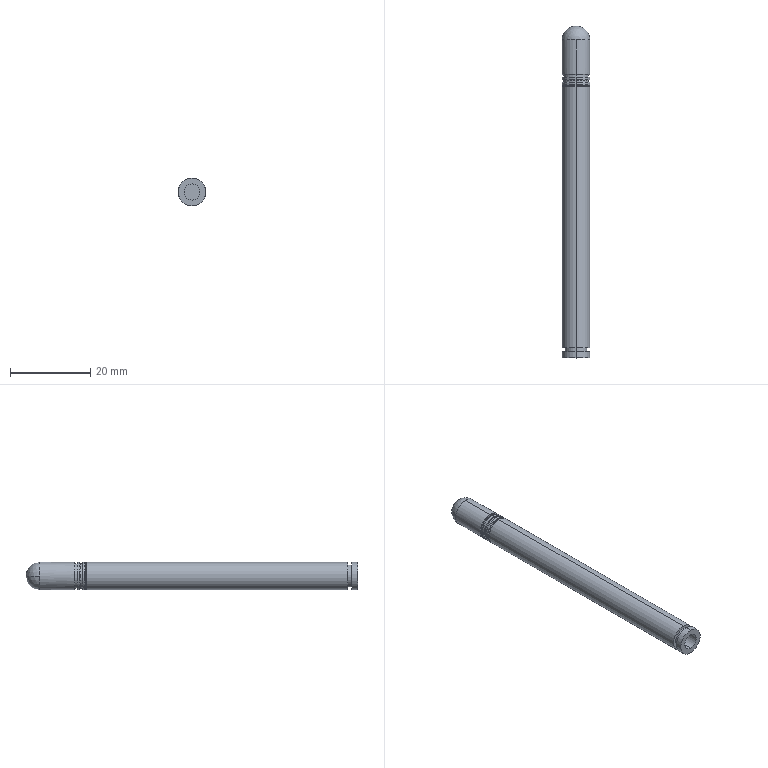Part | SolidWorks | features Revolution 1 | 1 solid | 56 faces | box 6.9 x 82.6 x 6.9 mm | volume 2024 mm3 | torus 24 | cylinder 20 | plane 10 | sphere 2 | commonest cylinder face diameters 6.9 x10 6.2 x6 4 x2 5.4 x2
STEP:
#1=CARTESIAN_POINT('',(0.,2.7,-2.7));
#2=VERTEX_POINT('',#1);
#3=CARTESIAN_POINT('',(0.,2.7,2.7));
#4=VERTEX_POINT('',#3);
#5=CARTESIAN_POINT('',(0.,2.7,0.));
#6=DIRECTION('',(0.,-1.,0.));
#7=DIRECTION('',(0.,0.,-1.));
#8=AXIS2_PLACEMENT_3D('',#5,#6,#7);
#9=CIRCLE('',#8,2.7);
#10=EDGE_CURVE('',#2,#4,#9,.T.);
#11=ORIENTED_EDGE('',*,*,#10,.T.);
#12=CARTESIAN_POINT('',(0.,1.7,2.7));
#13=VERTEX_POINT('',#12);
#14=CARTESIAN_POINT('',(0.,-7.874,2.7));
#15=DIRECTION('',(0.,-1.,0.));
#16=VECTOR('',#15,1000.);
#17=LINE('',#14,#16);
#18=EDGE_CURVE('',#4,#13,#17,.T.);
#19=ORIENTED_EDGE('',*,*,#18,.T.);
#20=CARTESIAN_POINT('',(0.,1.7,-2.7));
#21=VERTEX_POINT('',#20);
#22=CARTESIAN_POINT('',(0.,1.7,0.));
#23=DIRECTION('',(0.,-1.,0.));
#24=DIRECTION('',(0.,0.,-1.));
#25=AXIS2_PLACEMENT_3D('',#22,#23,#24);
#26=CIRCLE('',#25,2.7);
#27=EDGE_CURVE('',#21,#13,#26,.T.);
#28=ORIENTED_EDGE('',*,*,#27,.F.);
#29=CARTESIAN_POINT('',(0.,-7.874,-2.7));
#30=DIRECTION('',(0.,-1.,0.));
#31=VECTOR('',#30,1000.);
#32=LINE('',#29,#31);
#33=EDGE_CURVE('',#2,#21,#32,.T.);
#34=ORIENTED_EDGE('',*,*,#33,.F.);
#35=EDGE_LOOP('',(#11,#19,#28,#34));
#36=FACE_OUTER_BOUND('',#35,.T.);
#37=CARTESIAN_POINT('',(0.,-7.874,0.));
#38=DIRECTION('',(0.,-1.,0.));
#39=DIRECTION('',(0.,0.,-1.));
#40=AXIS2_PLACEMENT_3D('',#37,#38,#39);
#41=CYLINDRICAL_SURFACE('',#40,2.7);
#42=ADVANCED_FACE('',(#36),#41,.T.);
#43=CARTESIAN_POINT('',(0.,67.65,-3.45));
#44=VERTEX_POINT('',#43);
#45=CARTESIAN_POINT('',(0.,67.65,3.45));
#46=VERTEX_POINT('',#45);
#47=CARTESIAN_POINT('',(0.,67.65,0.));
#48=DIRECTION('',(0.,-1.,0.));
#49=DIRECTION('',(0.,0.,-1.));
#50=AXIS2_PLACEMENT_3D('',#47,#48,#49);
#51=CIRCLE('',#50,3.45);
#52=EDGE_CURVE('',#44,#46,#51,.T.);
#53=ORIENTED_EDGE('',*,*,#52,.T.);
#54=CARTESIAN_POINT('',(0.,2.7,3.45));
#55=VERTEX_POINT('',#54);
#56=CARTESIAN_POINT('',(0.,-7.874,3.45));
#57=DIRECTION('',(0.,-1.,0.));
#58=VECTOR('',#57,1000.);
#59=LINE('',#56,#58);
#60=EDGE_CURVE('',#46,#55,#59,.T.);
#61=ORIENTED_EDGE('',*,*,#60,.T.);
#62=CARTESIAN_POINT('',(0.,2.7,-3.45));
#63=VERTEX_POINT('',#62);
#64=CARTESIAN_POINT('',(0.,2.7,0.));
#65=DIRECTION('',(0.,-1.,0.));
#66=DIRECTION('',(0.,0.,-1.));
#67=AXIS2_PLACEMENT_3D('',#64,#65,#66);
#68=CIRCLE('',#67,3.45);
#69=EDGE_CURVE('',#63,#55,#68,.T.);
#70=ORIENTED_EDGE('',*,*,#69,.F.);
#71=CARTESIAN_POINT('',(0.,-7.874,-3.45));
#72=DIRECTION('',(0.,-1.,0.));
#73=VECTOR('',#72,1000.);
#74=LINE('',#71,#73);
#75=EDGE_CURVE('',#44,#63,#74,.T.);
#76=ORIENTED_EDGE('',*,*,#75,.F.);
#77=EDGE_LOOP('',(#53,#61,#70,#76));
#78=FACE_OUTER_BOUND('',#77,.T.);
#79=CARTESIAN_POINT('',(0.,-7.874,0.));
#80=DIRECTION('',(0.,-1.,0.));
#81=DIRECTION('',(0.,0.,-1.));
#82=AXIS2_PLACEMENT_3D('',#79,#80,#81);
#83=CYLINDRICAL_SURFACE('',#82,3.45);
#84=ADVANCED_FACE('',(#78),#83,.T.);
#85=CARTESIAN_POINT('',(0.,67.7,-3.4));
#86=VERTEX_POINT('',#85);
#87=CARTESIAN_POINT('',(0.,67.7,3.4));
#88=VERTEX_POINT('',#87);
#89=CARTESIAN_POINT('',(0.,67.7,0.));
#90=DIRECTION('',(0.,-1.,0.));
#91=DIRECTION('',(0.,0.,-1.));
#92=AXIS2_PLACEMENT_3D('',#89,#90,#91);
#93=CIRCLE('',#92,3.4);
#94=EDGE_CURVE('',#86,#88,#93,.T.);
#95=ORIENTED_EDGE('',*,*,#94,.T.);
#96=CARTESIAN_POINT('',(0.,67.65,3.4));
#97=DIRECTION('',(1.,0.,0.));
#98=DIRECTION('',(0.,0.,-1.));
#99=AXIS2_PLACEMENT_3D('',#96,#97,#98);
#100=CIRCLE('',#99,0.05);
#101=EDGE_CURVE('',#88,#46,#100,.T.);
#102=ORIENTED_EDGE('',*,*,#101,.T.);
#103=ORIENTED_EDGE('',*,*,#52,.F.);
#104=CARTESIAN_POINT('',(0.,67.65,-3.4));
#105=DIRECTION('',(-1.,0.,0.));
#106=DIRECTION('',(0.,0.,1.));
#107=AXIS2_PLACEMENT_3D('',#104,#105,#106);
#108=CIRCLE('',#107,0.05);
#109=EDGE_CURVE('',#86,#44,#108,.T.);
#110=ORIENTED_EDGE('',*,*,#109,.F.);
#111=EDGE_LOOP('',(#95,#102,#103,#110));
#112=FACE_OUTER_BOUND('',#111,.T.);
#113=CARTESIAN_POINT('',(0.,67.65,0.));
#114=DIRECTION('',(0.,-1.,0.));
#115=DIRECTION('',(0.,0.,-1.));
#116=AXIS2_PLACEMENT_3D('',#113,#114,#115);
#117=TOROIDAL_SURFACE('',#116,3.4,0.05);
#118=ADVANCED_FACE('',(#112),#117,.T.);
#119=CARTESIAN_POINT('',(0.,67.7,3.15));
#120=VERTEX_POINT('',#119);
#121=CARTESIAN_POINT('',(0.,67.7,-3.15));
#122=VERTEX_POINT('',#121);
#123=CARTESIAN_POINT('',(0.,67.7,0.));
#124=DIRECTION('',(0.,-1.,0.));
#125=DIRECTION('',(0.,0.,-1.));
#126=AXIS2_PLACEMENT_3D('',#123,#124,#125);
#127=CIRCLE('',#126,3.15);
#128=EDGE_CURVE('',#120,#122,#127,.T.);
#129=ORIENTED_EDGE('',*,*,#128,.F.);
#130=CARTESIAN_POINT('',(0.,67.75,3.1));
#131=VERTEX_POINT('',#130);
#132=CARTESIAN_POINT('',(0.,67.75,3.15));
#133=DIRECTION('',(1.,0.,0.));
#134=DIRECTION('',(0.,0.,-1.));
#135=AXIS2_PLACEMENT_3D('',#132,#133,#134);
#136=CIRCLE('',#135,0.05);
#137=EDGE_CURVE('',#120,#131,#136,.T.);
#138=ORIENTED_EDGE('',*,*,#137,.T.);
#139=CARTESIAN_POINT('',(0.,67.75,-3.1));
#140=VERTEX_POINT('',#139);
#141=CARTESIAN_POINT('',(0.,67.75,0.));
#142=DIRECTION('',(0.,-1.,0.));
#143=DIRECTION('',(0.,0.,-1.));
#144=AXIS2_PLACEMENT_3D('',#141,#142,#143);
#145=CIRCLE('',#144,3.1);
#146=EDGE_CURVE('',#131,#140,#145,.T.);
#147=ORIENTED_EDGE('',*,*,#146,.T.);
#148=CARTESIAN_POINT('',(0.,67.75,-3.15));
#149=DIRECTION('',(-1.,0.,0.));
#150=DIRECTION('',(0.,0.,1.));
#151=AXIS2_PLACEMENT_3D('',#148,#149,#150);
#152=CIRCLE('',#151,0.05);
#153=EDGE_CURVE('',#122,#140,#152,.T.);
#154=ORIENTED_EDGE('',*,*,#153,.F.);
#155=EDGE_LOOP('',(#129,#138,#147,#154));
#156=FACE_OUTER_BOUND('',#155,.T.);
#157=CARTESIAN_POINT('',(0.,67.75,0.));
#158=DIRECTION('',(0.,-1.,0.));
#159=DIRECTION('',(0.,0.,-1.));
#160=AXIS2_PLACEMENT_3D('',#157,#158,#159);
#161=TOROIDAL_SURFACE('',#160,3.15,0.05);
#162=ADVANCED_FACE('',(#156),#161,.F.);
#163=CARTESIAN_POINT('',(0.,68.05,-3.1));
#164=VERTEX_POINT('',#163);
#165=CARTESIAN_POINT('',(0.,68.05,3.1));
#166=VERTEX_POINT('',#165);
#167=CARTESIAN_POINT('',(0.,68.05,0.));
#168=DIRECTION('',(0.,-1.,0.));
#169=DIRECTION('',(0.,0.,-1.));
#170=AXIS2_PLACEMENT_3D('',#167,#168,#169);
#171=CIRCLE('',#170,3.1);
#172=EDGE_CURVE('',#164,#166,#171,.T.);
#173=ORIENTED_EDGE('',*,*,#172,.T.);
#174=CARTESIAN_POINT('',(0.,-7.874,3.1));
#175=DIRECTION('',(0.,-1.,0.));
#176=VECTOR('',#175,1000.);
#177=LINE('',#174,#176);
#178=EDGE_CURVE('',#166,#131,#177,.T.);
#179=ORIENTED_EDGE('',*,*,#178,.T.);
#180=CARTESIAN_POINT('',(0.,67.75,0.));
#181=DIRECTION('',(0.,-1.,0.));
#182=DIRECTION('',(0.,0.,-1.));
#183=AXIS2_PLACEMENT_3D('',#180,#181,#182);
#184=CIRCLE('',#183,3.1);
#185=EDGE_CURVE('',#140,#131,#184,.T.);
#186=ORIENTED_EDGE('',*,*,#185,.F.);
#187=CARTESIAN_POINT('',(0.,-7.874,-3.1));
#188=DIRECTION('',(0.,-1.,0.));
#189=VECTOR('',#188,1000.);
#190=LINE('',#187,#189);
#191=EDGE_CURVE('',#164,#140,#190,.T.);
#192=ORIENTED_EDGE('',*,*,#191,.F.);
#193=EDGE_LOOP('',(#173,#179,#186,#192));
#194=FACE_OUTER_BOUND('',#193,.T.);
#195=CARTESIAN_POINT('',(0.,-7.874,0.));
#196=DIRECTION('',(0.,-1.,0.));
#197=DIRECTION('',(0.,0.,-1.));
#198=AXIS2_PLACEMENT_3D('',#195,#196,#197);
#199=CYLINDRICAL_SURFACE('',#198,3.1);
#200=ADVANCED_FACE('',(#194),#199,.T.);
#201=CARTESIAN_POINT('',(0.,68.05,0.));
#202=DIRECTION('',(0.,-1.,0.));
#203=DIRECTION('',(0.,0.,-1.));
#204=AXIS2_PLACEMENT_3D('',#201,#202,#203);
#205=CIRCLE('',#204,3.1);
#206=EDGE_CURVE('',#166,#164,#205,.T.);
#207=ORIENTED_EDGE('',*,*,#206,.F.);
#208=CARTESIAN_POINT('',(0.,68.1,3.15));
#209=VERTEX_POINT('',#208);
#210=CARTESIAN_POINT('',(0.,68.05,3.15));
#211=DIRECTION('',(1.,0.,0.));
#212=DIRECTION('',(0.,0.,-1.));
#213=AXIS2_PLACEMENT_3D('',#210,#211,#212);
#214=CIRCLE('',#213,0.05);
#215=EDGE_CURVE('',#166,#209,#214,.T.);
#216=ORIENTED_EDGE('',*,*,#215,.T.);
#217=CARTESIAN_POINT('',(0.,68.1,-3.15));
#218=VERTEX_POINT('',#217);
#219=CARTESIAN_POINT('',(0.,68.1,0.));
#220=DIRECTION('',(0.,-1.,0.));
#221=DIRECTION('',(0.,0.,-1.));
#222=AXIS2_PLACEMENT_3D('',#219,#220,#221);
#223=CIRCLE('',#222,3.15);
#224=EDGE_CURVE('',#209,#218,#223,.T.);
#225=ORIENTED_EDGE('',*,*,#224,.T.);
#226=CARTESIAN_POINT('',(0.,68.05,-3.15));
#227=DIRECTION('',(-1.,0.,0.));
#228=DIRECTION('',(0.,0.,1.));
#229=AXIS2_PLACEMENT_3D('',#226,#227,#228);
#230=CIRCLE('',#229,0.05);
#231=EDGE_CURVE('',#164,#218,#230,.T.);
#232=ORIENTED_EDGE('',*,*,#231,.F.);
#233=EDGE_LOOP('',(#207,#216,#225,#232));
#234=FACE_OUTER_BOUND('',#233,.T.);
#235=CARTESIAN_POINT('',(0.,68.05,0.));
#236=DIRECTION('',(0.,-1.,0.));
#237=DIRECTION('',(0.,0.,-1.));
#238=AXIS2_PLACEMENT_3D('',#235,#236,#237);
#239=TOROIDAL_SURFACE('',#238,3.15,0.05);
#240=ADVANCED_FACE('',(#234),#239,.F.);
#241=CARTESIAN_POINT('',(0.,68.15,-3.45));
#242=VERTEX_POINT('',#241);
#243=CARTESIAN_POINT('',(0.,68.15,3.45));
#244=VERTEX_POINT('',#243);
#245=CARTESIAN_POINT('',(0.,68.15,0.));
#246=DIRECTION('',(0.,-1.,0.));
#247=DIRECTION('',(0.,0.,-1.));
#248=AXIS2_PLACEMENT_3D('',#245,#246,#247);
#249=CIRCLE('',#248,3.45);
#250=EDGE_CURVE('',#242,#244,#249,.T.);
#251=ORIENTED_EDGE('',*,*,#250,.T.);
#252=CARTESIAN_POINT('',(0.,68.1,3.4));
#253=VERTEX_POINT('',#252);
#254=CARTESIAN_POINT('',(0.,68.15,3.4));
#255=DIRECTION('',(1.,0.,0.));
#256=DIRECTION('',(0.,0.,-1.));
#257=AXIS2_PLACEMENT_3D('',#254,#255,#256);
#258=CIRCLE('',#257,0.05);
#259=EDGE_CURVE('',#244,#253,#258,.T.);
#260=ORIENTED_EDGE('',*,*,#259,.T.);
#261=CARTESIAN_POINT('',(0.,68.1,-3.4));
#262=VERTEX_POINT('',#261);
#263=CARTESIAN_POINT('',(0.,68.1,0.));
#264=DIRECTION('',(0.,-1.,0.));
#265=DIRECTION('',(0.,0.,-1.));
#266=AXIS2_PLACEMENT_3D('',#263,#264,#265);
#267=CIRCLE('',#266,3.4);
#268=EDGE_CURVE('',#262,#253,#267,.T.);
#269=ORIENTED_EDGE('',*,*,#268,.F.);
#270=CARTESIAN_POINT('',(0.,68.15,-3.4));
#271=DIRECTION('',(-1.,0.,0.));
#272=DIRECTION('',(0.,0.,1.));
#273=AXIS2_PLACEMENT_3D('',#270,#271,#272);
#274=CIRCLE('',#273,0.05);
#275=EDGE_CURVE('',#242,#262,#274,.T.);
#276=ORIENTED_EDGE('',*,*,#275,.F.);
#277=EDGE_LOOP('',(#251,#260,#269,#276));
#278=FACE_OUTER_BOUND('',#277,.T.);
#279=CARTESIAN_POINT('',(0.,68.15,0.));
#280=DIRECTION('',(0.,-1.,0.));
#281=DIRECTION('',(0.,0.,-1.));
#282=AXIS2_PLACEMENT_3D('',#279,#280,#281);
#283=TOROIDAL_SURFACE('',#282,3.4,0.05);
#284=ADVANCED_FACE('',(#278),#283,.T.);
#285=CARTESIAN_POINT('',(0.,68.7,-3.45));
#286=VERTEX_POINT('',#285);
#287=CARTESIAN_POINT('',(0.,68.7,3.45));
#288=VERTEX_POINT('',#287);
#289=CARTESIAN_POINT('',(0.,68.7,0.));
#290=DIRECTION('',(0.,-1.,0.));
#291=DIRECTION('',(0.,0.,-1.));
#292=AXIS2_PLACEMENT_3D('',#289,#290,#291);
#293=CIRCLE('',#292,3.45);
#294=EDGE_CURVE('',#286,#288,#293,.T.);
#295=ORIENTED_EDGE('',*,*,#294,.T.);
#296=CARTESIAN_POINT('',(0.,-7.874,3.45));
#297=DIRECTION('',(0.,-1.,0.));
#298=VECTOR('',#297,1000.);
#299=LINE('',#296,#298);
#300=EDGE_CURVE('',#288,#244,#299,.T.);
#301=ORIENTED_EDGE('',*,*,#300,.T.);
#302=ORIENTED_EDGE('',*,*,#250,.F.);
#303=CARTESIAN_POINT('',(0.,-7.874,-3.45));
#304=DIRECTION('',(0.,-1.,0.));
#305=VECTOR('',#304,1000.);
#306=LINE('',#303,#305);
#307=EDGE_CURVE('',#286,#242,#306,.T.);
#308=ORIENTED_EDGE('',*,*,#307,.F.);
#309=EDGE_LOOP('',(#295,#301,#302,#308));
#310=FACE_OUTER_BOUND('',#309,.T.);
#311=CARTESIAN_POINT('',(0.,-7.874,0.));
#312=DIRECTION('',(0.,-1.,0.));
#313=DIRECTION('',(0.,0.,-1.));
#314=AXIS2_PLACEMENT_3D('',#311,#312,#313);
#315=CYLINDRICAL_SURFACE('',#314,3.45);
#316=ADVANCED_FACE('',(#310),#315,.T.);
#317=CARTESIAN_POINT('',(0.,68.75,-3.4));
#318=VERTEX_POINT('',#317);
#319=CARTESIAN_POINT('',(0.,68.75,3.4));
#320=VERTEX_POINT('',#319);
#321=CARTESIAN_POINT('',(0.,68.75,0.));
#322=DIRECTION('',(0.,-1.,0.));
#323=DIRECTION('',(0.,0.,-1.));
#324=AXIS2_PLACEMENT_3D('',#321,#322,#323);
#325=CIRCLE('',#324,3.4);
#326=EDGE_CURVE('',#318,#320,#325,.T.);
#327=ORIENTED_EDGE('',*,*,#326,.T.);
#328=CARTESIAN_POINT('',(0.,68.7,3.4));
#329=DIRECTION('',(1.,0.,0.));
#330=DIRECTION('',(0.,0.,-1.));
#331=AXIS2_PLACEMENT_3D('',#328,#329,#330);
#332=CIRCLE('',#331,0.05);
#333=EDGE_CURVE('',#320,#288,#332,.T.);
#334=ORIENTED_EDGE('',*,*,#333,.T.);
#335=ORIENTED_EDGE('',*,*,#294,.F.);
#336=CARTESIAN_POINT('',(0.,68.7,-3.4));
#337=DIRECTION('',(-1.,0.,0.));
#338=DIRECTION('',(0.,0.,1.));
#339=AXIS2_PLACEMENT_3D('',#336,#337,#338);
#340=CIRCLE('',#339,0.05);
#341=EDGE_CURVE('',#318,#286,#340,.T.);
#342=ORIENTED_EDGE('',*,*,#341,.F.);
#343=EDGE_LOOP('',(#327,#334,#335,#342));
#344=FACE_OUTER_BOUND('',#343,.T.);
#345=CARTESIAN_POINT('',(0.,68.7,0.));
#346=DIRECTION('',(0.,-1.,0.));
#347=DIRECTION('',(0.,0.,-1.));
#348=AXIS2_PLACEMENT_3D('',#345,#346,#347);
#349=TOROIDAL_SURFACE('',#348,3.4,0.05);
#350=ADVANCED_FACE('',(#344),#349,.T.);
#351=CARTESIAN_POINT('',(0.,68.75,3.15));
#352=VERTEX_POINT('',#351);
#353=CARTESIAN_POINT('',(0.,68.75,-3.15));
#354=VERTEX_POINT('',#353);
#355=CARTESIAN_POINT('',(0.,68.75,0.));
#356=DIRECTION('',(0.,-1.,0.));
#357=DIRECTION('',(0.,0.,-1.));
#358=AXIS2_PLACEMENT_3D('',#355,#356,#357);
#359=CIRCLE('',#358,3.15);
#360=EDGE_CURVE('',#352,#354,#359,.T.);
#361=ORIENTED_EDGE('',*,*,#360,.F.);
#362=CARTESIAN_POINT('',(0.,68.8,3.1));
#363=VERTEX_POINT('',#362);
#364=CARTESIAN_POINT('',(0.,68.8,3.15));
#365=DIRECTION('',(1.,0.,0.));
#366=DIRECTION('',(0.,0.,-1.));
#367=AXIS2_PLACEMENT_3D('',#364,#365,#366);
#368=CIRCLE('',#367,0.05);
#369=EDGE_CURVE('',#352,#363,#368,.T.);
#370=ORIENTED_EDGE('',*,*,#369,.T.);
#371=CARTESIAN_POINT('',(0.,68.8,-3.1));
#372=VERTEX_POINT('',#371);
#373=CARTESIAN_POINT('',(0.,68.8,0.));
#374=DIRECTION('',(0.,-1.,0.));
#375=DIRECTION('',(0.,0.,-1.));
#376=AXIS2_PLACEMENT_3D('',#373,#374,#375);
#377=CIRCLE('',#376,3.1);
#378=EDGE_CURVE('',#363,#372,#377,.T.);
#379=ORIENTED_EDGE('',*,*,#378,.T.);
#380=CARTESIAN_POINT('',(0.,68.8,-3.15));
#381=DIRECTION('',(-1.,0.,0.));
#382=DIRECTION('',(0.,0.,1.));
#383=AXIS2_PLACEMENT_3D('',#380,#381,#382);
#384=CIRCLE('',#383,0.05);
#385=EDGE_CURVE('',#354,#372,#384,.T.);
#386=ORIENTED_EDGE('',*,*,#385,.F.);
#387=EDGE_LOOP('',(#361,#370,#379,#386));
#388=FACE_OUTER_BOUND('',#387,.T.);
#389=CARTESIAN_POINT('',(0.,68.8,0.));
#390=DIRECTION('',(0.,-1.,0.));
#391=DIRECTION('',(0.,0.,-1.));
#392=AXIS2_PLACEMENT_3D('',#389,#390,#391);
#393=TOROIDAL_SURFACE('',#392,3.15,0.05);
#394=ADVANCED_FACE('',(#388),#393,.F.);
#395=CARTESIAN_POINT('',(0.,69.35,-3.1));
#396=VERTEX_POINT('',#395);
#397=CARTESIAN_POINT('',(0.,69.35,3.1));
#398=VERTEX_POINT('',#397);
#399=CARTESIAN_POINT('',(0.,69.35,0.));
#400=DIRECTION('',(0.,-1.,0.));
#401=DIRECTION('',(0.,0.,-1.));
#402=AXIS2_PLACEMENT_3D('',#399,#400,#401);
#403=CIRCLE('',#402,3.1);
#404=EDGE_CURVE('',#396,#398,#403,.T.);
#405=ORIENTED_EDGE('',*,*,#404,.T.);
#406=CARTESIAN_POINT('',(0.,-7.874,3.1));
#407=DIRECTION('',(0.,-1.,0.));
#408=VECTOR('',#407,1000.);
#409=LINE('',#406,#408);
#410=EDGE_CURVE('',#398,#363,#409,.T.);
#411=ORIENTED_EDGE('',*,*,#410,.T.);
#412=CARTESIAN_POINT('',(0.,68.8,0.));
#413=DIRECTION('',(0.,-1.,0.));
#414=DIRECTION('',(0.,0.,-1.));
#415=AXIS2_PLACEMENT_3D('',#412,#413,#414);
#416=CIRCLE('',#415,3.1);
#417=EDGE_CURVE('',#372,#363,#416,.T.);
#418=ORIENTED_EDGE('',*,*,#417,.F.);
#419=CARTESIAN_POINT('',(0.,-7.874,-3.1));
#420=DIRECTION('',(0.,-1.,0.));
#421=VECTOR('',#420,1000.);
#422=LINE('',#419,#421);
#423=EDGE_CURVE('',#396,#372,#422,.T.);
#424=ORIENTED_EDGE('',*,*,#423,.F.);
#425=EDGE_LOOP('',(#405,#411,#418,#424));
#426=FACE_OUTER_BOUND('',#425,.T.);
#427=CARTESIAN_POINT('',(0.,-7.874,0.));
#428=DIRECTION('',(0.,-1.,0.));
#429=DIRECTION('',(0.,0.,-1.));
#430=AXIS2_PLACEMENT_3D('',#427,#428,#429);
#431=CYLINDRICAL_SURFACE('',#430,3.1);
#432=ADVANCED_FACE('',(#426),#431,.T.);
#433=CARTESIAN_POINT('',(0.,69.35,0.));
#434=DIRECTION('',(0.,-1.,0.));
#435=DIRECTION('',(0.,0.,-1.));
#436=AXIS2_PLACEMENT_3D('',#433,#434,#435);
#437=CIRCLE('',#436,3.1);
#438=EDGE_CURVE('',#398,#396,#437,.T.);
#439=ORIENTED_EDGE('',*,*,#438,.F.);
#440=CARTESIAN_POINT('',(0.,69.4,3.15));
#441=VERTEX_POINT('',#440);
#442=CARTESIAN_POINT('',(0.,69.35,3.15));
#443=DIRECTION('',(1.,0.,0.));
#444=DIRECTION('',(0.,0.,-1.));
#445=AXIS2_PLACEMENT_3D('',#442,#443,#444);
#446=CIRCLE('',#445,0.05);
#447=EDGE_CURVE('',#398,#441,#446,.T.);
#448=ORIENTED_EDGE('',*,*,#447,.T.);
#449=CARTESIAN_POINT('',(0.,69.4,-3.15));
#450=VERTEX_POINT('',#449);
#451=CARTESIAN_POINT('',(0.,69.4,0.));
#452=DIRECTION('',(0.,-1.,0.));
#453=DIRECTION('',(0.,0.,-1.));
#454=AXIS2_PLACEMENT_3D('',#451,#452,#453);
#455=CIRCLE('',#454,3.15);
#456=EDGE_CURVE('',#441,#450,#455,.T.);
#457=ORIENTED_EDGE('',*,*,#456,.T.);
#458=CARTESIAN_POINT('',(0.,69.35,-3.15));
#459=DIRECTION('',(-1.,0.,0.));
#460=DIRECTION('',(0.,0.,1.));
#461=AXIS2_PLACEMENT_3D('',#458,#459,#460);
#462=CIRCLE('',#461,0.05);
#463=EDGE_CURVE('',#396,#450,#462,.T.);
#464=ORIENTED_EDGE('',*,*,#463,.F.);
#465=EDGE_LOOP('',(#439,#448,#457,#464));
#466=FACE_OUTER_BOUND('',#465,.T.);
#467=CARTESIAN_POINT('',(0.,69.35,0.));
#468=DIRECTION('',(0.,-1.,0.));
#469=DIRECTION('',(0.,0.,-1.));
#470=AXIS2_PLACEMENT_3D('',#467,#468,#469);
#471=TOROIDAL_SURFACE('',#470,3.15,0.05);
#472=ADVANCED_FACE('',(#466),#471,.F.);
#473=CARTESIAN_POINT('',(0.,69.45,-3.45));
#474=VERTEX_POINT('',#473);
#475=CARTESIAN_POINT('',(0.,69.45,3.45));
#476=VERTEX_POINT('',#475);
#477=CARTESIAN_POINT('',(0.,69.45,0.));
#478=DIRECTION('',(0.,-1.,0.));
#479=DIRECTION('',(0.,0.,-1.));
#480=AXIS2_PLACEMENT_3D('',#477,#478,#479);
#481=CIRCLE('',#480,3.45);
#482=EDGE_CURVE('',#474,#476,#481,.T.);
#483=ORIENTED_EDGE('',*,*,#482,.T.);
#484=CARTESIAN_POINT('',(0.,69.4,3.4));
#485=VERTEX_POINT('',#484);
#486=CARTESIAN_POINT('',(0.,69.45,3.4));
#487=DIRECTION('',(1.,0.,0.));
#488=DIRECTION('',(0.,0.,-1.));
#489=AXIS2_PLACEMENT_3D('',#486,#487,#488);
#490=CIRCLE('',#489,0.05);
#491=EDGE_CURVE('',#476,#485,#490,.T.);
#492=ORIENTED_EDGE('',*,*,#491,.T.);
#493=CARTESIAN_POINT('',(0.,69.4,-3.4));
#494=VERTEX_POINT('',#493);
#495=CARTESIAN_POINT('',(0.,69.4,0.));
#496=DIRECTION('',(0.,-1.,0.));
#497=DIRECTION('',(0.,0.,-1.));
#498=AXIS2_PLACEMENT_3D('',#495,#496,#497);
#499=CIRCLE('',#498,3.4);
#500=EDGE_CURVE('',#494,#485,#499,.T.);
#501=ORIENTED_EDGE('',*,*,#500,.F.);
#502=CARTESIAN_POINT('',(0.,69.45,-3.4));
#503=DIRECTION('',(-1.,0.,0.));
#504=DIRECTION('',(0.,0.,1.));
#505=AXIS2_PLACEMENT_3D('',#502,#503,#504);
#506=CIRCLE('',#505,0.05);
#507=EDGE_CURVE('',#474,#494,#506,.T.);
#508=ORIENTED_EDGE('',*,*,#507,.F.);
#509=EDGE_LOOP('',(#483,#492,#501,#508));
#510=FACE_OUTER_BOUND('',#509,.T.);
#511=CARTESIAN_POINT('',(0.,69.45,0.));
#512=DIRECTION('',(0.,-1.,0.));
#513=DIRECTION('',(0.,0.,-1.));
#514=AXIS2_PLACEMENT_3D('',#511,#512,#513);
#515=TOROIDAL_SURFACE('',#514,3.4,0.05);
#516=ADVANCED_FACE('',(#510),#515,.T.);
#517=CARTESIAN_POINT('',(0.,70.,-3.45));
#518=VERTEX_POINT('',#517);
#519=CARTESIAN_POINT('',(0.,70.,3.45));
#520=VERTEX_POINT('',#519);
#521=CARTESIAN_POINT('',(0.,70.,0.));
#522=DIRECTION('',(0.,-1.,0.));
#523=DIRECTION('',(0.,0.,-1.));
#524=AXIS2_PLACEMENT_3D('',#521,#522,#523);
#525=CIRCLE('',#524,3.45);
#526=EDGE_CURVE('',#518,#520,#525,.T.);
#527=ORIENTED_EDGE('',*,*,#526,.T.);
#528=CARTESIAN_POINT('',(0.,-7.874,3.45));
#529=DIRECTION('',(0.,-1.,0.));
#530=VECTOR('',#529,1000.);
#531=LINE('',#528,#530);
#532=EDGE_CURVE('',#520,#476,#531,.T.);
#533=ORIENTED_EDGE('',*,*,#532,.T.);
#534=ORIENTED_EDGE('',*,*,#482,.F.);
#535=CARTESIAN_POINT('',(0.,-7.874,-3.45));
#536=DIRECTION('',(0.,-1.,0.));
#537=VECTOR('',#536,1000.);
#538=LINE('',#535,#537);
#539=EDGE_CURVE('',#518,#474,#538,.T.);
#540=ORIENTED_EDGE('',*,*,#539,.F.);
#541=EDGE_LOOP('',(#527,#533,#534,#540));
#542=FACE_OUTER_BOUND('',#541,.T.);
#543=CARTESIAN_POINT('',(0.,-7.874,0.));
#544=DIRECTION('',(0.,-1.,0.));
#545=DIRECTION('',(0.,0.,-1.));
#546=AXIS2_PLACEMENT_3D('',#543,#544,#545);
#547=CYLINDRICAL_SURFACE('',#546,3.45);
#548=ADVANCED_FACE('',(#542),#547,.T.);
#549=CARTESIAN_POINT('',(0.,70.05,-3.4));
#550=VERTEX_POINT('',#549);
#551=CARTESIAN_POINT('',(0.,70.05,3.4));
#552=VERTEX_POINT('',#551);
#553=CARTESIAN_POINT('',(0.,70.05,0.));
#554=DIRECTION('',(0.,-1.,0.));
#555=DIRECTION('',(0.,0.,-1.));
#556=AXIS2_PLACEMENT_3D('',#553,#554,#555);
#557=CIRCLE('',#556,3.4);
#558=EDGE_CURVE('',#550,#552,#557,.T.);
#559=ORIENTED_EDGE('',*,*,#558,.T.);
#560=CARTESIAN_POINT('',(0.,70.,3.4));
#561=DIRECTION('',(1.,0.,0.));
#562=DIRECTION('',(0.,0.,-1.));
#563=AXIS2_PLACEMENT_3D('',#560,#561,#562);
#564=CIRCLE('',#563,0.05);
#565=EDGE_CURVE('',#552,#520,#564,.T.);
#566=ORIENTED_EDGE('',*,*,#565,.T.);
#567=ORIENTED_EDGE('',*,*,#526,.F.);
#568=CARTESIAN_POINT('',(0.,70.,-3.4));
#569=DIRECTION('',(-1.,0.,0.));
#570=DIRECTION('',(0.,0.,1.));
#571=AXIS2_PLACEMENT_3D('',#568,#569,#570);
#572=CIRCLE('',#571,0.05);
#573=EDGE_CURVE('',#550,#518,#572,.T.);
#574=ORIENTED_EDGE('',*,*,#573,.F.);
#575=EDGE_LOOP('',(#559,#566,#567,#574));
#576=FACE_OUTER_BOUND('',#575,.T.);
#577=CARTESIAN_POINT('',(0.,70.,0.));
#578=DIRECTION('',(0.,-1.,0.));
#579=DIRECTION('',(0.,0.,-1.));
#580=AXIS2_PLACEMENT_3D('',#577,#578,#579);
#581=TOROIDAL_SURFACE('',#580,3.4,0.05);
#582=ADVANCED_FACE('',(#576),#581,.T.);
#583=CARTESIAN_POINT('',(0.,70.05,3.15));
#584=VERTEX_POINT('',#583);
#585=CARTESIAN_POINT('',(0.,70.05,-3.15));
#586=VERTEX_POINT('',#585);
#587=CARTESIAN_POINT('',(0.,70.05,0.));
#588=DIRECTION('',(0.,-1.,0.));
#589=DIRECTION('',(0.,0.,-1.));
#590=AXIS2_PLACEMENT_3D('',#587,#588,#589);
#591=CIRCLE('',#590,3.15);
#592=EDGE_CURVE('',#584,#586,#591,.T.);
#593=ORIENTED_EDGE('',*,*,#592,.F.);
#594=CARTESIAN_POINT('',(0.,70.1,3.1));
#595=VERTEX_POINT('',#594);
#596=CARTESIAN_POINT('',(0.,70.1,3.15));
#597=DIRECTION('',(1.,0.,0.));
#598=DIRECTION('',(0.,0.,-1.));
#599=AXIS2_PLACEMENT_3D('',#596,#597,#598);
#600=CIRCLE('',#599,0.05);
#601=EDGE_CURVE('',#584,#595,#600,.T.);
#602=ORIENTED_EDGE('',*,*,#601,.T.);
#603=CARTESIAN_POINT('',(0.,70.1,-3.1));
#604=VERTEX_POINT('',#603);
#605=CARTESIAN_POINT('',(0.,70.1,0.));
#606=DIRECTION('',(0.,-1.,0.));
#607=DIRECTION('',(0.,0.,-1.));
#608=AXIS2_PLACEMENT_3D('',#605,#606,#607);
#609=CIRCLE('',#608,3.1);
#610=EDGE_CURVE('',#595,#604,#609,.T.);
#611=ORIENTED_EDGE('',*,*,#610,.T.);
#612=CARTESIAN_POINT('',(0.,70.1,-3.15));
#613=DIRECTION('',(-1.,0.,0.));
#614=DIRECTION('',(0.,0.,1.));
#615=AXIS2_PLACEMENT_3D('',#612,#613,#614);
#616=CIRCLE('',#615,0.05);
#617=EDGE_CURVE('',#586,#604,#616,.T.);
#618=ORIENTED_EDGE('',*,*,#617,.F.);
#619=EDGE_LOOP('',(#593,#602,#611,#618));
#620=FACE_OUTER_BOUND('',#619,.T.);
#621=CARTESIAN_POINT('',(0.,70.1,0.));
#622=DIRECTION('',(0.,-1.,0.));
#623=DIRECTION('',(0.,0.,-1.));
#624=AXIS2_PLACEMENT_3D('',#621,#622,#623);
#625=TOROIDAL_SURFACE('',#624,3.15,0.05);
#626=ADVANCED_FACE('',(#620),#625,.F.);
#627=CARTESIAN_POINT('',(0.,70.65,-3.1));
#628=VERTEX_POINT('',#627);
#629=CARTESIAN_POINT('',(0.,70.65,3.1));
#630=VERTEX_POINT('',#629);
#631=CARTESIAN_POINT('',(0.,70.65,0.));
#632=DIRECTION('',(0.,-1.,0.));
#633=DIRECTION('',(0.,0.,-1.));
#634=AXIS2_PLACEMENT_3D('',#631,#632,#633);
#635=CIRCLE('',#634,3.1);
#636=EDGE_CURVE('',#628,#630,#635,.T.);
#637=ORIENTED_EDGE('',*,*,#636,.T.);
#638=CARTESIAN_POINT('',(0.,-7.874,3.1));
#639=DIRECTION('',(0.,-1.,0.));
#640=VECTOR('',#639,1000.);
#641=LINE('',#638,#640);
#642=EDGE_CURVE('',#630,#595,#641,.T.);
#643=ORIENTED_EDGE('',*,*,#642,.T.);
#644=CARTESIAN_POINT('',(0.,70.1,0.));
#645=DIRECTION('',(0.,-1.,0.));
#646=DIRECTION('',(0.,0.,-1.));
#647=AXIS2_PLACEMENT_3D('',#644,#645,#646);
#648=CIRCLE('',#647,3.1);
#649=EDGE_CURVE('',#604,#595,#648,.T.);
#650=ORIENTED_EDGE('',*,*,#649,.F.);
#651=CARTESIAN_POINT('',(0.,-7.874,-3.1));
#652=DIRECTION('',(0.,-1.,0.));
#653=VECTOR('',#652,1000.);
#654=LINE('',#651,#653);
#655=EDGE_CURVE('',#628,#604,#654,.T.);
#656=ORIENTED_EDGE('',*,*,#655,.F.);
#657=EDGE_LOOP('',(#637,#643,#650,#656));
#658=FACE_OUTER_BOUND('',#657,.T.);
#659=CARTESIAN_POINT('',(0.,-7.874,0.));
#660=DIRECTION('',(0.,-1.,0.));
#661=DIRECTION('',(0.,0.,-1.));
#662=AXIS2_PLACEMENT_3D('',#659,#660,#661);
#663=CYLINDRICAL_SURFACE('',#662,3.1);
#664=ADVANCED_FACE('',(#658),#663,.T.);
#665=CARTESIAN_POINT('',(0.,70.65,0.));
#666=DIRECTION('',(0.,-1.,0.));
#667=DIRECTION('',(0.,0.,-1.));
#668=AXIS2_PLACEMENT_3D('',#665,#666,#667);
#669=CIRCLE('',#668,3.1);
#670=EDGE_CURVE('',#630,#628,#669,.T.);
#671=ORIENTED_EDGE('',*,*,#670,.F.);
#672=CARTESIAN_POINT('',(0.,70.7,3.15));
#673=VERTEX_POINT('',#672);
#674=CARTESIAN_POINT('',(0.,70.65,3.15));
#675=DIRECTION('',(1.,0.,0.));
#676=DIRECTION('',(0.,0.,-1.));
#677=AXIS2_PLACEMENT_3D('',#674,#675,#676);
#678=CIRCLE('',#677,0.05);
#679=EDGE_CURVE('',#630,#673,#678,.T.);
#680=ORIENTED_EDGE('',*,*,#679,.T.);
#681=CARTESIAN_POINT('',(0.,70.7,-3.15));
#682=VERTEX_POINT('',#681);
#683=CARTESIAN_POINT('',(0.,70.7,0.));
#684=DIRECTION('',(0.,-1.,0.));
#685=DIRECTION('',(0.,0.,-1.));
#686=AXIS2_PLACEMENT_3D('',#683,#684,#685);
#687=CIRCLE('',#686,3.15);
#688=EDGE_CURVE('',#673,#682,#687,.T.);
#689=ORIENTED_EDGE('',*,*,#688,.T.);
#690=CARTESIAN_POINT('',(0.,70.65,-3.15));
#691=DIRECTION('',(-1.,0.,0.));
#692=DIRECTION('',(0.,0.,1.));
#693=AXIS2_PLACEMENT_3D('',#690,#691,#692);
#694=CIRCLE('',#693,0.05);
#695=EDGE_CURVE('',#628,#682,#694,.T.);
#696=ORIENTED_EDGE('',*,*,#695,.F.);
#697=EDGE_LOOP('',(#671,#680,#689,#696));
#698=FACE_OUTER_BOUND('',#697,.T.);
#699=CARTESIAN_POINT('',(0.,70.65,0.));
#700=DIRECTION('',(0.,-1.,0.));
#701=DIRECTION('',(0.,0.,-1.));
#702=AXIS2_PLACEMENT_3D('',#699,#700,#701);
#703=TOROIDAL_SURFACE('',#702,3.15,0.05);
#704=ADVANCED_FACE('',(#698),#703,.F.);
#705=CARTESIAN_POINT('',(0.,70.75,-3.45));
#706=VERTEX_POINT('',#705);
#707=CARTESIAN_POINT('',(0.,70.75,3.45));
#708=VERTEX_POINT('',#707);
#709=CARTESIAN_POINT('',(0.,70.75,0.));
#710=DIRECTION('',(0.,-1.,0.));
#711=DIRECTION('',(0.,0.,-1.));
#712=AXIS2_PLACEMENT_3D('',#709,#710,#711);
#713=CIRCLE('',#712,3.45);
#714=EDGE_CURVE('',#706,#708,#713,.T.);
#715=ORIENTED_EDGE('',*,*,#714,.T.);
#716=CARTESIAN_POINT('',(0.,70.7,3.4));
#717=VERTEX_POINT('',#716);
#718=CARTESIAN_POINT('',(0.,70.75,3.4));
#719=DIRECTION('',(1.,0.,0.));
#720=DIRECTION('',(0.,0.,-1.));
#721=AXIS2_PLACEMENT_3D('',#718,#719,#720);
#722=CIRCLE('',#721,0.05);
#723=EDGE_CURVE('',#708,#717,#722,.T.);
#724=ORIENTED_EDGE('',*,*,#723,.T.);
#725=CARTESIAN_POINT('',(0.,70.7,-3.4));
#726=VERTEX_POINT('',#725);
#727=CARTESIAN_POINT('',(0.,70.7,0.));
#728=DIRECTION('',(0.,-1.,0.));
#729=DIRECTION('',(0.,0.,-1.));
#730=AXIS2_PLACEMENT_3D('',#727,#728,#729);
#731=CIRCLE('',#730,3.4);
#732=EDGE_CURVE('',#726,#717,#731,.T.);
#733=ORIENTED_EDGE('',*,*,#732,.F.);
#734=CARTESIAN_POINT('',(0.,70.75,-3.4));
#735=DIRECTION('',(-1.,0.,0.));
#736=DIRECTION('',(0.,0.,1.));
#737=AXIS2_PLACEMENT_3D('',#734,#735,#736);
#738=CIRCLE('',#737,0.05);
#739=EDGE_CURVE('',#706,#726,#738,.T.);
#740=ORIENTED_EDGE('',*,*,#739,.F.);
#741=EDGE_LOOP('',(#715,#724,#733,#740));
#742=FACE_OUTER_BOUND('',#741,.T.);
#743=CARTESIAN_POINT('',(0.,70.75,0.));
#744=DIRECTION('',(0.,-1.,0.));
#745=DIRECTION('',(0.,0.,-1.));
#746=AXIS2_PLACEMENT_3D('',#743,#744,#745);
#747=TOROIDAL_SURFACE('',#746,3.4,0.05);
#748=ADVANCED_FACE('',(#742),#747,.T.);
#749=CARTESIAN_POINT('',(3.45,79.35,0.));
#750=VERTEX_POINT('',#749);
#751=CARTESIAN_POINT('',(0.,79.35,3.45));
#752=VERTEX_POINT('',#751);
#753=CARTESIAN_POINT('',(0.,79.35,0.));
#754=DIRECTION('',(0.,-1.,0.));
#755=DIRECTION('',(0.,0.,-1.));
#756=AXIS2_PLACEMENT_3D('',#753,#754,#755);
#757=CIRCLE('',#756,3.45);
#758=EDGE_CURVE('',#750,#752,#757,.T.);
#759=ORIENTED_EDGE('',*,*,#758,.T.);
#760=CARTESIAN_POINT('',(0.,-7.874,3.45));
#761=DIRECTION('',(0.,-1.,0.));
#762=VECTOR('',#761,1000.);
#763=LINE('',#760,#762);
#764=EDGE_CURVE('',#752,#708,#763,.T.);
#765=ORIENTED_EDGE('',*,*,#764,.T.);
#766=ORIENTED_EDGE('',*,*,#714,.F.);
#767=CARTESIAN_POINT('',(0.,79.35,-3.45));
#768=VERTEX_POINT('',#767);
#769=CARTESIAN_POINT('',(0.,-7.874,-3.45));
#770=DIRECTION('',(0.,-1.,0.));
#771=VECTOR('',#770,1000.);
#772=LINE('',#769,#771);
#773=EDGE_CURVE('',#768,#706,#772,.T.);
#774=ORIENTED_EDGE('',*,*,#773,.F.);
#775=CARTESIAN_POINT('',(0.,79.35,0.));
#776=DIRECTION('',(0.,-1.,0.));
#777=DIRECTION('',(0.,0.,-1.));
#778=AXIS2_PLACEMENT_3D('',#775,#776,#777);
#779=CIRCLE('',#778,3.45);
#780=EDGE_CURVE('',#768,#750,#779,.T.);
#781=ORIENTED_EDGE('',*,*,#780,.T.);
#782=EDGE_LOOP('',(#759,#765,#766,#774,#781));
#783=FACE_OUTER_BOUND('',#782,.T.);
#784=CARTESIAN_POINT('',(0.,-7.874,0.));
#785=DIRECTION('',(0.,-1.,0.));
#786=DIRECTION('',(0.,0.,-1.));
#787=AXIS2_PLACEMENT_3D('',#784,#785,#786);
#788=CYLINDRICAL_SURFACE('',#787,3.45);
#789=ADVANCED_FACE('',(#783),#788,.T.);
#790=CARTESIAN_POINT('',(0.,82.8,0.));
#791=VERTEX_POINT('',#790);
#792=CARTESIAN_POINT('',(0.,79.35,0.));
#793=DIRECTION('',(0.,0.,-1.));
#794=DIRECTION('',(-1.,0.,0.));
#795=AXIS2_PLACEMENT_3D('',#792,#793,#794);
#796=CIRCLE('',#795,3.45);
#797=EDGE_CURVE('',#791,#750,#796,.T.);
#798=ORIENTED_EDGE('',*,*,#797,.F.);
#799=CARTESIAN_POINT('',(-3.45,79.35,0.));
#800=VERTEX_POINT('',#799);
#801=CARTESIAN_POINT('',(0.,79.35,0.));
#802=DIRECTION('',(0.,0.,1.));
#803=DIRECTION('',(1.,0.,0.));
#804=AXIS2_PLACEMENT_3D('',#801,#802,#803);
#805=CIRCLE('',#804,3.45);
#806=EDGE_CURVE('',#791,#800,#805,.T.);
#807=ORIENTED_EDGE('',*,*,#806,.T.);
#808=CARTESIAN_POINT('',(0.,79.35,0.));
#809=DIRECTION('',(0.,-1.,0.));
#810=DIRECTION('',(0.,0.,-1.));
#811=AXIS2_PLACEMENT_3D('',#808,#809,#810);
#812=CIRCLE('',#811,3.45);
#813=EDGE_CURVE('',#752,#800,#812,.T.);
#814=ORIENTED_EDGE('',*,*,#813,.F.);
#815=ORIENTED_EDGE('',*,*,#758,.F.);
#816=EDGE_LOOP('',(#798,#807,#814,#815));
#817=FACE_OUTER_BOUND('',#816,.T.);
#818=CARTESIAN_POINT('',(0.,79.35,0.));
#819=DIRECTION('',(0.,0.,1.));
#820=DIRECTION('',(1.,0.,0.));
#821=AXIS2_PLACEMENT_3D('',#818,#819,#820);
#822=SPHERICAL_SURFACE('',#821,3.45);
#823=ADVANCED_FACE('',(#817),#822,.T.);
#824=CARTESIAN_POINT('',(0.,79.35,2.));
#825=VERTEX_POINT('',#824);
#826=CARTESIAN_POINT('',(0.,79.35,-2.));
#827=VERTEX_POINT('',#826);
#828=CARTESIAN_POINT('',(0.,79.35,0.));
#829=DIRECTION('',(0.,-1.,0.));
#830=DIRECTION('',(0.,0.,-1.));
#831=AXIS2_PLACEMENT_3D('',#828,#829,#830);
#832=CIRCLE('',#831,2.);
#833=EDGE_CURVE('',#825,#827,#832,.T.);
#834=ORIENTED_EDGE('',*,*,#833,.F.);
#835=CARTESIAN_POINT('',(0.,0.2,2.));
#836=VERTEX_POINT('',#835);
#837=CARTESIAN_POINT('',(0.,-7.874,2.));
#838=DIRECTION('',(0.,-1.,0.));
#839=VECTOR('',#838,1000.);
#840=LINE('',#837,#839);
#841=EDGE_CURVE('',#825,#836,#840,.T.);
#842=ORIENTED_EDGE('',*,*,#841,.T.);
#843=CARTESIAN_POINT('',(0.,0.2,-2.));
#844=VERTEX_POINT('',#843);
#845=CARTESIAN_POINT('',(0.,0.2,0.));
#846=DIRECTION('',(0.,-1.,0.));
#847=DIRECTION('',(0.,0.,-1.));
#848=AXIS2_PLACEMENT_3D('',#845,#846,#847);
#849=CIRCLE('',#848,2.);
#850=EDGE_CURVE('',#836,#844,#849,.T.);
#851=ORIENTED_EDGE('',*,*,#850,.T.);
#852=CARTESIAN_POINT('',(0.,-7.874,-2.));
#853=DIRECTION('',(0.,-1.,0.));
#854=VECTOR('',#853,1000.);
#855=LINE('',#852,#854);
#856=EDGE_CURVE('',#827,#844,#855,.T.);
#857=ORIENTED_EDGE('',*,*,#856,.F.);
#858=EDGE_LOOP('',(#834,#842,#851,#857));
#859=FACE_OUTER_BOUND('',#858,.T.);
#860=CARTESIAN_POINT('',(0.,-7.874,0.));
#861=DIRECTION('',(0.,-1.,0.));
#862=DIRECTION('',(0.,0.,-1.));
#863=AXIS2_PLACEMENT_3D('',#860,#861,#862);
#864=CYLINDRICAL_SURFACE('',#863,2.);
#865=ADVANCED_FACE('',(#859),#864,.F.);
#866=CARTESIAN_POINT('',(0.,1.7,-3.45));
#867=VERTEX_POINT('',#866);
#868=CARTESIAN_POINT('',(0.,1.7,3.45));
#869=VERTEX_POINT('',#868);
#870=CARTESIAN_POINT('',(0.,1.7,0.));
#871=DIRECTION('',(0.,-1.,0.));
#872=DIRECTION('',(0.,0.,-1.));
#873=AXIS2_PLACEMENT_3D('',#870,#871,#872);
#874=CIRCLE('',#873,3.45);
#875=EDGE_CURVE('',#867,#869,#874,.T.);
#876=ORIENTED_EDGE('',*,*,#875,.T.);
#877=CARTESIAN_POINT('',(0.,0.2,3.45));
#878=VERTEX_POINT('',#877);
#879=CARTESIAN_POINT('',(0.,-7.874,3.45));
#880=DIRECTION('',(0.,-1.,0.));
#881=VECTOR('',#880,1000.);
#882=LINE('',#879,#881);
#883=EDGE_CURVE('',#869,#878,#882,.T.);
#884=ORIENTED_EDGE('',*,*,#883,.T.);
#885=CARTESIAN_POINT('',(0.,0.2,-3.45));
#886=VERTEX_POINT('',#885);
#887=CARTESIAN_POINT('',(0.,0.2,0.));
#888=DIRECTION('',(0.,-1.,0.));
#889=DIRECTION('',(0.,0.,-1.));
#890=AXIS2_PLACEMENT_3D('',#887,#888,#889);
#891=CIRCLE('',#890,3.45);
#892=EDGE_CURVE('',#886,#878,#891,.T.);
#893=ORIENTED_EDGE('',*,*,#892,.F.);
#894=CARTESIAN_POINT('',(0.,-7.874,-3.45));
#895=DIRECTION('',(0.,-1.,0.));
#896=VECTOR('',#895,1000.);
#897=LINE('',#894,#896);
#898=EDGE_CURVE('',#867,#886,#897,.T.);
#899=ORIENTED_EDGE('',*,*,#898,.F.);
#900=EDGE_LOOP('',(#876,#884,#893,#899));
#901=FACE_OUTER_BOUND('',#900,.T.);
#902=CARTESIAN_POINT('',(0.,-7.874,0.));
#903=DIRECTION('',(0.,-1.,0.));
#904=DIRECTION('',(0.,0.,-1.));
#905=AXIS2_PLACEMENT_3D('',#902,#903,#904);
#906=CYLINDRICAL_SURFACE('',#905,3.45);
#907=ADVANCED_FACE('',(#901),#906,.T.);
#908=ORIENTED_EDGE('',*,*,#883,.F.);
#909=CARTESIAN_POINT('',(0.,1.7,0.));
#910=DIRECTION('',(0.,-1.,0.));
#911=DIRECTION('',(0.,0.,-1.));
#912=AXIS2_PLACEMENT_3D('',#909,#910,#911);
#913=CIRCLE('',#912,3.45);
#914=EDGE_CURVE('',#869,#867,#913,.T.);
#915=ORIENTED_EDGE('',*,*,#914,.T.);
#916=ORIENTED_EDGE('',*,*,#898,.T.);
#917=CARTESIAN_POINT('',(0.,0.2,0.));
#918=DIRECTION('',(0.,-1.,0.));
#919=DIRECTION('',(0.,0.,-1.));
#920=AXIS2_PLACEMENT_3D('',#917,#918,#919);
#921=CIRCLE('',#920,3.45);
#922=EDGE_CURVE('',#878,#886,#921,.T.);
#923=ORIENTED_EDGE('',*,*,#922,.F.);
#924=EDGE_LOOP('',(#908,#915,#916,#923));
#925=FACE_OUTER_BOUND('',#924,.T.);
#926=CARTESIAN_POINT('',(0.,-7.874,0.));
#927=DIRECTION('',(0.,-1.,0.));
#928=DIRECTION('',(0.,0.,-1.));
#929=AXIS2_PLACEMENT_3D('',#926,#927,#928);
#930=CYLINDRICAL_SURFACE('',#929,3.45);
#931=ADVANCED_FACE('',(#925),#930,.T.);
#932=ORIENTED_EDGE('',*,*,#892,.T.);
#933=ORIENTED_EDGE('',*,*,#922,.T.);
#934=EDGE_LOOP('',(#932,#933));
#935=FACE_OUTER_BOUND('',#934,.T.);
#936=CARTESIAN_POINT('',(0.,0.2,0.));
#937=DIRECTION('',(0.,-1.,0.));
#938=DIRECTION('',(0.,0.,-1.));
#939=AXIS2_PLACEMENT_3D('',#936,#937,#938);
#940=CIRCLE('',#939,2.);
#941=EDGE_CURVE('',#844,#836,#940,.T.);
#942=ORIENTED_EDGE('',*,*,#941,.F.);
#943=ORIENTED_EDGE('',*,*,#850,.F.);
#944=EDGE_LOOP('',(#942,#943));
#945=FACE_BOUND('',#944,.T.);
#946=CARTESIAN_POINT('',(2.,0.2,0.));
#947=DIRECTION('',(0.,-1.,0.));
#948=DIRECTION('',(0.,0.,-1.));
#949=AXIS2_PLACEMENT_3D('',#946,#947,#948);
#950=PLANE('',#949);
#951=ADVANCED_FACE('',(#935,#945),#950,.T.);
#952=ORIENTED_EDGE('',*,*,#841,.F.);
#953=CARTESIAN_POINT('',(0.,79.35,0.));
#954=DIRECTION('',(0.,-1.,0.));
#955=DIRECTION('',(0.,0.,-1.));
#956=AXIS2_PLACEMENT_3D('',#953,#954,#955);
#957=CIRCLE('',#956,2.);
#958=EDGE_CURVE('',#827,#825,#957,.T.);
#959=ORIENTED_EDGE('',*,*,#958,.F.);
#960=ORIENTED_EDGE('',*,*,#856,.T.);
#961=ORIENTED_EDGE('',*,*,#941,.T.);
#962=EDGE_LOOP('',(#952,#959,#960,#961));
#963=FACE_OUTER_BOUND('',#962,.T.);
#964=CARTESIAN_POINT('',(0.,-7.874,0.));
#965=DIRECTION('',(0.,-1.,0.));
#966=DIRECTION('',(0.,0.,-1.));
#967=AXIS2_PLACEMENT_3D('',#964,#965,#966);
#968=CYLINDRICAL_SURFACE('',#967,2.);
#969=ADVANCED_FACE('',(#963),#968,.F.);
#970=ORIENTED_EDGE('',*,*,#958,.T.);
#971=ORIENTED_EDGE('',*,*,#833,.T.);
#972=EDGE_LOOP('',(#970,#971));
#973=FACE_OUTER_BOUND('',#972,.T.);
#974=CARTESIAN_POINT('',(2.,79.35,0.));
#975=DIRECTION('',(0.,-1.,0.));
#976=DIRECTION('',(0.,0.,-1.));
#977=AXIS2_PLACEMENT_3D('',#974,#975,#976);
#978=PLANE('',#977);
#979=ADVANCED_FACE('',(#973),#978,.T.);
#980=ORIENTED_EDGE('',*,*,#806,.F.);
#981=ORIENTED_EDGE('',*,*,#797,.T.);
#982=ORIENTED_EDGE('',*,*,#780,.F.);
#983=CARTESIAN_POINT('',(0.,79.35,0.));
#984=DIRECTION('',(0.,-1.,0.));
#985=DIRECTION('',(0.,0.,-1.));
#986=AXIS2_PLACEMENT_3D('',#983,#984,#985);
#987=CIRCLE('',#986,3.45);
#988=EDGE_CURVE('',#800,#768,#987,.T.);
#989=ORIENTED_EDGE('',*,*,#988,.F.);
#990=EDGE_LOOP('',(#980,#981,#982,#989));
#991=FACE_OUTER_BOUND('',#990,.T.);
#992=CARTESIAN_POINT('',(0.,79.35,0.));
#993=DIRECTION('',(0.,0.,1.));
#994=DIRECTION('',(1.,0.,0.));
#995=AXIS2_PLACEMENT_3D('',#992,#993,#994);
#996=SPHERICAL_SURFACE('',#995,3.45);
#997=ADVANCED_FACE('',(#991),#996,.T.);
#998=ORIENTED_EDGE('',*,*,#764,.F.);
#999=ORIENTED_EDGE('',*,*,#813,.T.);
#1000=ORIENTED_EDGE('',*,*,#988,.T.);
#1001=ORIENTED_EDGE('',*,*,#773,.T.);
#1002=CARTESIAN_POINT('',(0.,70.75,0.));
#1003=DIRECTION('',(0.,-1.,0.));
#1004=DIRECTION('',(0.,0.,-1.));
#1005=AXIS2_PLACEMENT_3D('',#1002,#1003,#1004);
#1006=CIRCLE('',#1005,3.45);
#1007=EDGE_CURVE('',#708,#706,#1006,.T.);
#1008=ORIENTED_EDGE('',*,*,#1007,.F.);
#1009=EDGE_LOOP('',(#998,#999,#1000,#1001,#1008));
#1010=FACE_OUTER_BOUND('',#1009,.T.);
#1011=CARTESIAN_POINT('',(0.,-7.874,0.));
#1012=DIRECTION('',(0.,-1.,0.));
#1013=DIRECTION('',(0.,0.,-1.));
#1014=AXIS2_PLACEMENT_3D('',#1011,#1012,#1013);
#1015=CYLINDRICAL_SURFACE('',#1014,3.45);
#1016=ADVANCED_FACE('',(#1010),#1015,.T.);
#1017=ORIENTED_EDGE('',*,*,#723,.F.);
#1018=ORIENTED_EDGE('',*,*,#1007,.T.);
#1019=ORIENTED_EDGE('',*,*,#739,.T.);
#1020=CARTESIAN_POINT('',(0.,70.7,0.));
#1021=DIRECTION('',(0.,-1.,0.));
#1022=DIRECTION('',(0.,0.,-1.));
#1023=AXIS2_PLACEMENT_3D('',#1020,#1021,#1022);
#1024=CIRCLE('',#1023,3.4);
#1025=EDGE_CURVE('',#717,#726,#1024,.T.);
#1026=ORIENTED_EDGE('',*,*,#1025,.F.);
#1027=EDGE_LOOP('',(#1017,#1018,#1019,#1026));
#1028=FACE_OUTER_BOUND('',#1027,.T.);
#1029=CARTESIAN_POINT('',(0.,70.75,0.));
#1030=DIRECTION('',(0.,-1.,0.));
#1031=DIRECTION('',(0.,0.,-1.));
#1032=AXIS2_PLACEMENT_3D('',#1029,#1030,#1031);
#1033=TOROIDAL_SURFACE('',#1032,3.4,0.05);
#1034=ADVANCED_FACE('',(#1028),#1033,.T.);
#1035=ORIENTED_EDGE('',*,*,#732,.T.);
#1036=ORIENTED_EDGE('',*,*,#1025,.T.);
#1037=EDGE_LOOP('',(#1035,#1036));
#1038=FACE_OUTER_BOUND('',#1037,.T.);
#1039=CARTESIAN_POINT('',(0.,70.7,0.));
#1040=DIRECTION('',(0.,-1.,0.));
#1041=DIRECTION('',(0.,0.,-1.));
#1042=AXIS2_PLACEMENT_3D('',#1039,#1040,#1041);
#1043=CIRCLE('',#1042,3.15);
#1044=EDGE_CURVE('',#682,#673,#1043,.T.);
#1045=ORIENTED_EDGE('',*,*,#1044,.F.);
#1046=ORIENTED_EDGE('',*,*,#688,.F.);
#1047=EDGE_LOOP('',(#1045,#1046));
#1048=FACE_BOUND('',#1047,.T.);
#1049=CARTESIAN_POINT('',(3.15,70.7,0.));
#1050=DIRECTION('',(0.,-1.,0.));
#1051=DIRECTION('',(0.,0.,-1.));
#1052=AXIS2_PLACEMENT_3D('',#1049,#1050,#1051);
#1053=PLANE('',#1052);
#1054=ADVANCED_FACE('',(#1038,#1048),#1053,.T.);
#1055=ORIENTED_EDGE('',*,*,#679,.F.);
#1056=ORIENTED_EDGE('',*,*,#636,.F.);
#1057=ORIENTED_EDGE('',*,*,#695,.T.);
#1058=ORIENTED_EDGE('',*,*,#1044,.T.);
#1059=EDGE_LOOP('',(#1055,#1056,#1057,#1058));
#1060=FACE_OUTER_BOUND('',#1059,.T.);
#1061=CARTESIAN_POINT('',(0.,70.65,0.));
#1062=DIRECTION('',(0.,-1.,0.));
#1063=DIRECTION('',(0.,0.,-1.));
#1064=AXIS2_PLACEMENT_3D('',#1061,#1062,#1063);
#1065=TOROIDAL_SURFACE('',#1064,3.15,0.05);
#1066=ADVANCED_FACE('',(#1060),#1065,.F.);
#1067=ORIENTED_EDGE('',*,*,#642,.F.);
#1068=ORIENTED_EDGE('',*,*,#670,.T.);
#1069=ORIENTED_EDGE('',*,*,#655,.T.);
#1070=ORIENTED_EDGE('',*,*,#610,.F.);
#1071=EDGE_LOOP('',(#1067,#1068,#1069,#1070));
#1072=FACE_OUTER_BOUND('',#1071,.T.);
#1073=CARTESIAN_POINT('',(0.,-7.874,0.));
#1074=DIRECTION('',(0.,-1.,0.));
#1075=DIRECTION('',(0.,0.,-1.));
#1076=AXIS2_PLACEMENT_3D('',#1073,#1074,#1075);
#1077=CYLINDRICAL_SURFACE('',#1076,3.1);
#1078=ADVANCED_FACE('',(#1072),#1077,.T.);
#1079=ORIENTED_EDGE('',*,*,#601,.F.);
#1080=CARTESIAN_POINT('',(0.,70.05,0.));
#1081=DIRECTION('',(0.,-1.,0.));
#1082=DIRECTION('',(0.,0.,-1.));
#1083=AXIS2_PLACEMENT_3D('',#1080,#1081,#1082);
#1084=CIRCLE('',#1083,3.15);
#1085=EDGE_CURVE('',#586,#584,#1084,.T.);
#1086=ORIENTED_EDGE('',*,*,#1085,.F.);
#1087=ORIENTED_EDGE('',*,*,#617,.T.);
#1088=ORIENTED_EDGE('',*,*,#649,.T.);
#1089=EDGE_LOOP('',(#1079,#1086,#1087,#1088));
#1090=FACE_OUTER_BOUND('',#1089,.T.);
#1091=CARTESIAN_POINT('',(0.,70.1,0.));
#1092=DIRECTION('',(0.,-1.,0.));
#1093=DIRECTION('',(0.,0.,-1.));
#1094=AXIS2_PLACEMENT_3D('',#1091,#1092,#1093);
#1095=TOROIDAL_SURFACE('',#1094,3.15,0.05);
#1096=ADVANCED_FACE('',(#1090),#1095,.F.);
#1097=ORIENTED_EDGE('',*,*,#1085,.T.);
#1098=ORIENTED_EDGE('',*,*,#592,.T.);
#1099=EDGE_LOOP('',(#1097,#1098));
#1100=FACE_BOUND('',#1099,.T.);
#1101=ORIENTED_EDGE('',*,*,#558,.F.);
#1102=CARTESIAN_POINT('',(0.,70.05,0.));
#1103=DIRECTION('',(0.,-1.,0.));
#1104=DIRECTION('',(0.,0.,-1.));
#1105=AXIS2_PLACEMENT_3D('',#1102,#1103,#1104);
#1106=CIRCLE('',#1105,3.4);
#1107=EDGE_CURVE('',#552,#550,#1106,.T.);
#1108=ORIENTED_EDGE('',*,*,#1107,.F.);
#1109=EDGE_LOOP('',(#1101,#1108));
#1110=FACE_OUTER_BOUND('',#1109,.T.);
#1111=CARTESIAN_POINT('',(3.15,70.05,0.));
#1112=DIRECTION('',(0.,1.,0.));
#1113=DIRECTION('',(0.,0.,1.));
#1114=AXIS2_PLACEMENT_3D('',#1111,#1112,#1113);
#1115=PLANE('',#1114);
#1116=ADVANCED_FACE('',(#1100,#1110),#1115,.T.);
#1117=ORIENTED_EDGE('',*,*,#565,.F.);
#1118=ORIENTED_EDGE('',*,*,#1107,.T.);
#1119=ORIENTED_EDGE('',*,*,#573,.T.);
#1120=CARTESIAN_POINT('',(0.,70.,0.));
#1121=DIRECTION('',(0.,-1.,0.));
#1122=DIRECTION('',(0.,0.,-1.));
#1123=AXIS2_PLACEMENT_3D('',#1120,#1121,#1122);
#1124=CIRCLE('',#1123,3.45);
#1125=EDGE_CURVE('',#520,#518,#1124,.T.);
#1126=ORIENTED_EDGE('',*,*,#1125,.F.);
#1127=EDGE_LOOP('',(#1117,#1118,#1119,#1126));
#1128=FACE_OUTER_BOUND('',#1127,.T.);
#1129=CARTESIAN_POINT('',(0.,70.,0.));
#1130=DIRECTION('',(0.,-1.,0.));
#1131=DIRECTION('',(0.,0.,-1.));
#1132=AXIS2_PLACEMENT_3D('',#1129,#1130,#1131);
#1133=TOROIDAL_SURFACE('',#1132,3.4,0.05);
#1134=ADVANCED_FACE('',(#1128),#1133,.T.);
#1135=ORIENTED_EDGE('',*,*,#532,.F.);
#1136=ORIENTED_EDGE('',*,*,#1125,.T.);
#1137=ORIENTED_EDGE('',*,*,#539,.T.);
#1138=CARTESIAN_POINT('',(0.,69.45,0.));
#1139=DIRECTION('',(0.,-1.,0.));
#1140=DIRECTION('',(0.,0.,-1.));
#1141=AXIS2_PLACEMENT_3D('',#1138,#1139,#1140);
#1142=CIRCLE('',#1141,3.45);
#1143=EDGE_CURVE('',#476,#474,#1142,.T.);
#1144=ORIENTED_EDGE('',*,*,#1143,.F.);
#1145=EDGE_LOOP('',(#1135,#1136,#1137,#1144));
#1146=FACE_OUTER_BOUND('',#1145,.T.);
#1147=CARTESIAN_POINT('',(0.,-7.874,0.));
#1148=DIRECTION('',(0.,-1.,0.));
#1149=DIRECTION('',(0.,0.,-1.));
#1150=AXIS2_PLACEMENT_3D('',#1147,#1148,#1149);
#1151=CYLINDRICAL_SURFACE('',#1150,3.45);
#1152=ADVANCED_FACE('',(#1146),#1151,.T.);
#1153=ORIENTED_EDGE('',*,*,#491,.F.);
#1154=ORIENTED_EDGE('',*,*,#1143,.T.);
#1155=ORIENTED_EDGE('',*,*,#507,.T.);
#1156=CARTESIAN_POINT('',(0.,69.4,0.));
#1157=DIRECTION('',(0.,-1.,0.));
#1158=DIRECTION('',(0.,0.,-1.));
#1159=AXIS2_PLACEMENT_3D('',#1156,#1157,#1158);
#1160=CIRCLE('',#1159,3.4);
#1161=EDGE_CURVE('',#485,#494,#1160,.T.);
#1162=ORIENTED_EDGE('',*,*,#1161,.F.);
#1163=EDGE_LOOP('',(#1153,#1154,#1155,#1162));
#1164=FACE_OUTER_BOUND('',#1163,.T.);
#1165=CARTESIAN_POINT('',(0.,69.45,0.));
#1166=DIRECTION('',(0.,-1.,0.));
#1167=DIRECTION('',(0.,0.,-1.));
#1168=AXIS2_PLACEMENT_3D('',#1165,#1166,#1167);
#1169=TOROIDAL_SURFACE('',#1168,3.4,0.05);
#1170=ADVANCED_FACE('',(#1164),#1169,.T.);
#1171=ORIENTED_EDGE('',*,*,#500,.T.);
#1172=ORIENTED_EDGE('',*,*,#1161,.T.);
#1173=EDGE_LOOP('',(#1171,#1172));
#1174=FACE_OUTER_BOUND('',#1173,.T.);
#1175=CARTESIAN_POINT('',(0.,69.4,0.));
#1176=DIRECTION('',(0.,-1.,0.));
#1177=DIRECTION('',(0.,0.,-1.));
#1178=AXIS2_PLACEMENT_3D('',#1175,#1176,#1177);
#1179=CIRCLE('',#1178,3.15);
#1180=EDGE_CURVE('',#450,#441,#1179,.T.);
#1181=ORIENTED_EDGE('',*,*,#1180,.F.);
#1182=ORIENTED_EDGE('',*,*,#456,.F.);
#1183=EDGE_LOOP('',(#1181,#1182));
#1184=FACE_BOUND('',#1183,.T.);
#1185=CARTESIAN_POINT('',(3.15,69.4,0.));
#1186=DIRECTION('',(0.,-1.,0.));
#1187=DIRECTION('',(0.,0.,-1.));
#1188=AXIS2_PLACEMENT_3D('',#1185,#1186,#1187);
#1189=PLANE('',#1188);
#1190=ADVANCED_FACE('',(#1174,#1184),#1189,.T.);
#1191=ORIENTED_EDGE('',*,*,#447,.F.);
#1192=ORIENTED_EDGE('',*,*,#404,.F.);
#1193=ORIENTED_EDGE('',*,*,#463,.T.);
#1194=ORIENTED_EDGE('',*,*,#1180,.T.);
#1195=EDGE_LOOP('',(#1191,#1192,#1193,#1194));
#1196=FACE_OUTER_BOUND('',#1195,.T.);
#1197=CARTESIAN_POINT('',(0.,69.35,0.));
#1198=DIRECTION('',(0.,-1.,0.));
#1199=DIRECTION('',(0.,0.,-1.));
#1200=AXIS2_PLACEMENT_3D('',#1197,#1198,#1199);
#1201=TOROIDAL_SURFACE('',#1200,3.15,0.05);
#1202=ADVANCED_FACE('',(#1196),#1201,.F.);
#1203=ORIENTED_EDGE('',*,*,#410,.F.);
#1204=ORIENTED_EDGE('',*,*,#438,.T.);
#1205=ORIENTED_EDGE('',*,*,#423,.T.);
#1206=ORIENTED_EDGE('',*,*,#378,.F.);
#1207=EDGE_LOOP('',(#1203,#1204,#1205,#1206));
#1208=FACE_OUTER_BOUND('',#1207,.T.);
#1209=CARTESIAN_POINT('',(0.,-7.874,0.));
#1210=DIRECTION('',(0.,-1.,0.));
#1211=DIRECTION('',(0.,0.,-1.));
#1212=AXIS2_PLACEMENT_3D('',#1209,#1210,#1211);
#1213=CYLINDRICAL_SURFACE('',#1212,3.1);
#1214=ADVANCED_FACE('',(#1208),#1213,.T.);
#1215=ORIENTED_EDGE('',*,*,#369,.F.);
#1216=CARTESIAN_POINT('',(0.,68.75,0.));
#1217=DIRECTION('',(0.,-1.,0.));
#1218=DIRECTION('',(0.,0.,-1.));
#1219=AXIS2_PLACEMENT_3D('',#1216,#1217,#1218);
#1220=CIRCLE('',#1219,3.15);
#1221=EDGE_CURVE('',#354,#352,#1220,.T.);
#1222=ORIENTED_EDGE('',*,*,#1221,.F.);
#1223=ORIENTED_EDGE('',*,*,#385,.T.);
#1224=ORIENTED_EDGE('',*,*,#417,.T.);
#1225=EDGE_LOOP('',(#1215,#1222,#1223,#1224));
#1226=FACE_OUTER_BOUND('',#1225,.T.);
#1227=CARTESIAN_POINT('',(0.,68.8,0.));
#1228=DIRECTION('',(0.,-1.,0.));
#1229=DIRECTION('',(0.,0.,-1.));
#1230=AXIS2_PLACEMENT_3D('',#1227,#1228,#1229);
#1231=TOROIDAL_SURFACE('',#1230,3.15,0.05);
#1232=ADVANCED_FACE('',(#1226),#1231,.F.);
#1233=ORIENTED_EDGE('',*,*,#1221,.T.);
#1234=ORIENTED_EDGE('',*,*,#360,.T.);
#1235=EDGE_LOOP('',(#1233,#1234));
#1236=FACE_BOUND('',#1235,.T.);
#1237=ORIENTED_EDGE('',*,*,#326,.F.);
#1238=CARTESIAN_POINT('',(0.,68.75,0.));
#1239=DIRECTION('',(0.,-1.,0.));
#1240=DIRECTION('',(0.,0.,-1.));
#1241=AXIS2_PLACEMENT_3D('',#1238,#1239,#1240);
#1242=CIRCLE('',#1241,3.4);
#1243=EDGE_CURVE('',#320,#318,#1242,.T.);
#1244=ORIENTED_EDGE('',*,*,#1243,.F.);
#1245=EDGE_LOOP('',(#1237,#1244));
#1246=FACE_OUTER_BOUND('',#1245,.T.);
#1247=CARTESIAN_POINT('',(3.15,68.75,0.));
#1248=DIRECTION('',(0.,1.,0.));
#1249=DIRECTION('',(0.,0.,1.));
#1250=AXIS2_PLACEMENT_3D('',#1247,#1248,#1249);
#1251=PLANE('',#1250);
#1252=ADVANCED_FACE('',(#1236,#1246),#1251,.T.);
#1253=ORIENTED_EDGE('',*,*,#333,.F.);
#1254=ORIENTED_EDGE('',*,*,#1243,.T.);
#1255=ORIENTED_EDGE('',*,*,#341,.T.);
#1256=CARTESIAN_POINT('',(0.,68.7,0.));
#1257=DIRECTION('',(0.,-1.,0.));
#1258=DIRECTION('',(0.,0.,-1.));
#1259=AXIS2_PLACEMENT_3D('',#1256,#1257,#1258);
#1260=CIRCLE('',#1259,3.45);
#1261=EDGE_CURVE('',#288,#286,#1260,.T.);
#1262=ORIENTED_EDGE('',*,*,#1261,.F.);
#1263=EDGE_LOOP('',(#1253,#1254,#1255,#1262));
#1264=FACE_OUTER_BOUND('',#1263,.T.);
#1265=CARTESIAN_POINT('',(0.,68.7,0.));
#1266=DIRECTION('',(0.,-1.,0.));
#1267=DIRECTION('',(0.,0.,-1.));
#1268=AXIS2_PLACEMENT_3D('',#1265,#1266,#1267);
#1269=TOROIDAL_SURFACE('',#1268,3.4,0.05);
#1270=ADVANCED_FACE('',(#1264),#1269,.T.);
#1271=ORIENTED_EDGE('',*,*,#300,.F.);
#1272=ORIENTED_EDGE('',*,*,#1261,.T.);
#1273=ORIENTED_EDGE('',*,*,#307,.T.);
#1274=CARTESIAN_POINT('',(0.,68.15,0.));
#1275=DIRECTION('',(0.,-1.,0.));
#1276=DIRECTION('',(0.,0.,-1.));
#1277=AXIS2_PLACEMENT_3D('',#1274,#1275,#1276);
#1278=CIRCLE('',#1277,3.45);
#1279=EDGE_CURVE('',#244,#242,#1278,.T.);
#1280=ORIENTED_EDGE('',*,*,#1279,.F.);
#1281=EDGE_LOOP('',(#1271,#1272,#1273,#1280));
#1282=FACE_OUTER_BOUND('',#1281,.T.);
#1283=CARTESIAN_POINT('',(0.,-7.874,0.));
#1284=DIRECTION('',(0.,-1.,0.));
#1285=DIRECTION('',(0.,0.,-1.));
#1286=AXIS2_PLACEMENT_3D('',#1283,#1284,#1285);
#1287=CYLINDRICAL_SURFACE('',#1286,3.45);
#1288=ADVANCED_FACE('',(#1282),#1287,.T.);
#1289=ORIENTED_EDGE('',*,*,#259,.F.);
#1290=ORIENTED_EDGE('',*,*,#1279,.T.);
#1291=ORIENTED_EDGE('',*,*,#275,.T.);
#1292=CARTESIAN_POINT('',(0.,68.1,0.));
#1293=DIRECTION('',(0.,-1.,0.));
#1294=DIRECTION('',(0.,0.,-1.));
#1295=AXIS2_PLACEMENT_3D('',#1292,#1293,#1294);
#1296=CIRCLE('',#1295,3.4);
#1297=EDGE_CURVE('',#253,#262,#1296,.T.);
#1298=ORIENTED_EDGE('',*,*,#1297,.F.);
#1299=EDGE_LOOP('',(#1289,#1290,#1291,#1298));
#1300=FACE_OUTER_BOUND('',#1299,.T.);
#1301=CARTESIAN_POINT('',(0.,68.15,0.));
#1302=DIRECTION('',(0.,-1.,0.));
#1303=DIRECTION('',(0.,0.,-1.));
#1304=AXIS2_PLACEMENT_3D('',#1301,#1302,#1303);
#1305=TOROIDAL_SURFACE('',#1304,3.4,0.05);
#1306=ADVANCED_FACE('',(#1300),#1305,.T.);
#1307=ORIENTED_EDGE('',*,*,#268,.T.);
#1308=ORIENTED_EDGE('',*,*,#1297,.T.);
#1309=EDGE_LOOP('',(#1307,#1308));
#1310=FACE_OUTER_BOUND('',#1309,.T.);
#1311=CARTESIAN_POINT('',(0.,68.1,0.));
#1312=DIRECTION('',(0.,-1.,0.));
#1313=DIRECTION('',(0.,0.,-1.));
#1314=AXIS2_PLACEMENT_3D('',#1311,#1312,#1313);
#1315=CIRCLE('',#1314,3.15);
#1316=EDGE_CURVE('',#218,#209,#1315,.T.);
#1317=ORIENTED_EDGE('',*,*,#1316,.F.);
#1318=ORIENTED_EDGE('',*,*,#224,.F.);
#1319=EDGE_LOOP('',(#1317,#1318));
#1320=FACE_BOUND('',#1319,.T.);
#1321=CARTESIAN_POINT('',(3.15,68.1,0.));
#1322=DIRECTION('',(0.,-1.,0.));
#1323=DIRECTION('',(0.,0.,-1.));
#1324=AXIS2_PLACEMENT_3D('',#1321,#1322,#1323);
#1325=PLANE('',#1324);
#1326=ADVANCED_FACE('',(#1310,#1320),#1325,.T.);
#1327=ORIENTED_EDGE('',*,*,#215,.F.);
#1328=ORIENTED_EDGE('',*,*,#172,.F.);
#1329=ORIENTED_EDGE('',*,*,#231,.T.);
#1330=ORIENTED_EDGE('',*,*,#1316,.T.);
#1331=EDGE_LOOP('',(#1327,#1328,#1329,#1330));
#1332=FACE_OUTER_BOUND('',#1331,.T.);
#1333=CARTESIAN_POINT('',(0.,68.05,0.));
#1334=DIRECTION('',(0.,-1.,0.));
#1335=DIRECTION('',(0.,0.,-1.));
#1336=AXIS2_PLACEMENT_3D('',#1333,#1334,#1335);
#1337=TOROIDAL_SURFACE('',#1336,3.15,0.05);
#1338=ADVANCED_FACE('',(#1332),#1337,.F.);
#1339=ORIENTED_EDGE('',*,*,#178,.F.);
#1340=ORIENTED_EDGE('',*,*,#206,.T.);
#1341=ORIENTED_EDGE('',*,*,#191,.T.);
#1342=ORIENTED_EDGE('',*,*,#146,.F.);
#1343=EDGE_LOOP('',(#1339,#1340,#1341,#1342));
#1344=FACE_OUTER_BOUND('',#1343,.T.);
#1345=CARTESIAN_POINT('',(0.,-7.874,0.));
#1346=DIRECTION('',(0.,-1.,0.));
#1347=DIRECTION('',(0.,0.,-1.));
#1348=AXIS2_PLACEMENT_3D('',#1345,#1346,#1347);
#1349=CYLINDRICAL_SURFACE('',#1348,3.1);
#1350=ADVANCED_FACE('',(#1344),#1349,.T.);
#1351=ORIENTED_EDGE('',*,*,#137,.F.);
#1352=CARTESIAN_POINT('',(0.,67.7,0.));
#1353=DIRECTION('',(0.,-1.,0.));
#1354=DIRECTION('',(0.,0.,-1.));
#1355=AXIS2_PLACEMENT_3D('',#1352,#1353,#1354);
#1356=CIRCLE('',#1355,3.15);
#1357=EDGE_CURVE('',#122,#120,#1356,.T.);
#1358=ORIENTED_EDGE('',*,*,#1357,.F.);
#1359=ORIENTED_EDGE('',*,*,#153,.T.);
#1360=ORIENTED_EDGE('',*,*,#185,.T.);
#1361=EDGE_LOOP('',(#1351,#1358,#1359,#1360));
#1362=FACE_OUTER_BOUND('',#1361,.T.);
#1363=CARTESIAN_POINT('',(0.,67.75,0.));
#1364=DIRECTION('',(0.,-1.,0.));
#1365=DIRECTION('',(0.,0.,-1.));
#1366=AXIS2_PLACEMENT_3D('',#1363,#1364,#1365);
#1367=TOROIDAL_SURFACE('',#1366,3.15,0.05);
#1368=ADVANCED_FACE('',(#1362),#1367,.F.);
#1369=ORIENTED_EDGE('',*,*,#1357,.T.);
#1370=ORIENTED_EDGE('',*,*,#128,.T.);
#1371=EDGE_LOOP('',(#1369,#1370));
#1372=FACE_BOUND('',#1371,.T.);
#1373=ORIENTED_EDGE('',*,*,#94,.F.);
#1374=CARTESIAN_POINT('',(0.,67.7,0.));
#1375=DIRECTION('',(0.,-1.,0.));
#1376=DIRECTION('',(0.,0.,-1.));
#1377=AXIS2_PLACEMENT_3D('',#1374,#1375,#1376);
#1378=CIRCLE('',#1377,3.4);
#1379=EDGE_CURVE('',#88,#86,#1378,.T.);
#1380=ORIENTED_EDGE('',*,*,#1379,.F.);
#1381=EDGE_LOOP('',(#1373,#1380));
#1382=FACE_OUTER_BOUND('',#1381,.T.);
#1383=CARTESIAN_POINT('',(3.15,67.7,0.));
#1384=DIRECTION('',(0.,1.,0.));
#1385=DIRECTION('',(0.,0.,1.));
#1386=AXIS2_PLACEMENT_3D('',#1383,#1384,#1385);
#1387=PLANE('',#1386);
#1388=ADVANCED_FACE('',(#1372,#1382),#1387,.T.);
#1389=ORIENTED_EDGE('',*,*,#101,.F.);
#1390=ORIENTED_EDGE('',*,*,#1379,.T.);
#1391=ORIENTED_EDGE('',*,*,#109,.T.);
#1392=CARTESIAN_POINT('',(0.,67.65,0.));
#1393=DIRECTION('',(0.,-1.,0.));
#1394=DIRECTION('',(0.,0.,-1.));
#1395=AXIS2_PLACEMENT_3D('',#1392,#1393,#1394);
#1396=CIRCLE('',#1395,3.45);
#1397=EDGE_CURVE('',#46,#44,#1396,.T.);
#1398=ORIENTED_EDGE('',*,*,#1397,.F.);
#1399=EDGE_LOOP('',(#1389,#1390,#1391,#1398));
#1400=FACE_OUTER_BOUND('',#1399,.T.);
#1401=CARTESIAN_POINT('',(0.,67.65,0.));
#1402=DIRECTION('',(0.,-1.,0.));
#1403=DIRECTION('',(0.,0.,-1.));
#1404=AXIS2_PLACEMENT_3D('',#1401,#1402,#1403);
#1405=TOROIDAL_SURFACE('',#1404,3.4,0.05);
#1406=ADVANCED_FACE('',(#1400),#1405,.T.);
#1407=ORIENTED_EDGE('',*,*,#60,.F.);
#1408=ORIENTED_EDGE('',*,*,#1397,.T.);
#1409=ORIENTED_EDGE('',*,*,#75,.T.);
#1410=CARTESIAN_POINT('',(0.,2.7,0.));
#1411=DIRECTION('',(0.,-1.,0.));
#1412=DIRECTION('',(0.,0.,-1.));
#1413=AXIS2_PLACEMENT_3D('',#1410,#1411,#1412);
#1414=CIRCLE('',#1413,3.45);
#1415=EDGE_CURVE('',#55,#63,#1414,.T.);
#1416=ORIENTED_EDGE('',*,*,#1415,.F.);
#1417=EDGE_LOOP('',(#1407,#1408,#1409,#1416));
#1418=FACE_OUTER_BOUND('',#1417,.T.);
#1419=CARTESIAN_POINT('',(0.,-7.874,0.));
#1420=DIRECTION('',(0.,-1.,0.));
#1421=DIRECTION('',(0.,0.,-1.));
#1422=AXIS2_PLACEMENT_3D('',#1419,#1420,#1421);
#1423=CYLINDRICAL_SURFACE('',#1422,3.45);
#1424=ADVANCED_FACE('',(#1418),#1423,.T.);
#1425=ORIENTED_EDGE('',*,*,#69,.T.);
#1426=ORIENTED_EDGE('',*,*,#1415,.T.);
#1427=EDGE_LOOP('',(#1425,#1426));
#1428=FACE_OUTER_BOUND('',#1427,.T.);
#1429=ORIENTED_EDGE('',*,*,#10,.F.);
#1430=CARTESIAN_POINT('',(0.,2.7,0.));
#1431=DIRECTION('',(0.,-1.,0.));
#1432=DIRECTION('',(0.,0.,-1.));
#1433=AXIS2_PLACEMENT_3D('',#1430,#1431,#1432);
#1434=CIRCLE('',#1433,2.7);
#1435=EDGE_CURVE('',#4,#2,#1434,.T.);
#1436=ORIENTED_EDGE('',*,*,#1435,.F.);
#1437=EDGE_LOOP('',(#1429,#1436));
#1438=FACE_BOUND('',#1437,.T.);
#1439=CARTESIAN_POINT('',(3.45,2.7,0.));
#1440=DIRECTION('',(0.,-1.,0.));
#1441=DIRECTION('',(0.,0.,-1.));
#1442=AXIS2_PLACEMENT_3D('',#1439,#1440,#1441);
#1443=PLANE('',#1442);
#1444=ADVANCED_FACE('',(#1428,#1438),#1443,.T.);
#1445=ORIENTED_EDGE('',*,*,#18,.F.);
#1446=ORIENTED_EDGE('',*,*,#1435,.T.);
#1447=ORIENTED_EDGE('',*,*,#33,.T.);
#1448=CARTESIAN_POINT('',(0.,1.7,0.));
#1449=DIRECTION('',(0.,-1.,0.));
#1450=DIRECTION('',(0.,0.,-1.));
#1451=AXIS2_PLACEMENT_3D('',#1448,#1449,#1450);
#1452=CIRCLE('',#1451,2.7);
#1453=EDGE_CURVE('',#13,#21,#1452,.T.);
#1454=ORIENTED_EDGE('',*,*,#1453,.F.);
#1455=EDGE_LOOP('',(#1445,#1446,#1447,#1454));
#1456=FACE_OUTER_BOUND('',#1455,.T.);
#1457=CARTESIAN_POINT('',(0.,-7.874,0.));
#1458=DIRECTION('',(0.,-1.,0.));
#1459=DIRECTION('',(0.,0.,-1.));
#1460=AXIS2_PLACEMENT_3D('',#1457,#1458,#1459);
#1461=CYLINDRICAL_SURFACE('',#1460,2.7);
#1462=ADVANCED_FACE('',(#1456),#1461,.T.);
#1463=ORIENTED_EDGE('',*,*,#27,.T.);
#1464=ORIENTED_EDGE('',*,*,#1453,.T.);
#1465=EDGE_LOOP('',(#1463,#1464));
#1466=FACE_BOUND('',#1465,.T.);
#1467=ORIENTED_EDGE('',*,*,#875,.F.);
#1468=ORIENTED_EDGE('',*,*,#914,.F.);
#1469=EDGE_LOOP('',(#1467,#1468));
#1470=FACE_OUTER_BOUND('',#1469,.T.);
#1471=CARTESIAN_POINT('',(2.7,1.7,0.));
#1472=DIRECTION('',(0.,1.,0.));
#1473=DIRECTION('',(0.,0.,1.));
#1474=AXIS2_PLACEMENT_3D('',#1471,#1472,#1473);
#1475=PLANE('',#1474);
#1476=ADVANCED_FACE('',(#1466,#1470),#1475,.T.);
#1477=CLOSED_SHELL('',(#42,#84,#118,#162,#200,#240,#284,#316,#350,#394,#432,#472,#516,#548,#582,#626,#664,#704,#748,#789,#823,#865,#907,#931,#951,#969,#979,#997,#1016,#1034,#1054,#1066,#1078,#1096,#1116,#1134,#1152,#1170,#1190,#1202,#1214,#1232,#1252,#1270,#1288,#1306,#1326,#1338,#1350,#1368,#1388,#1406,#1424,#1444,#1462,#1476));
#1478=MANIFOLD_SOLID_BREP('',#1477);
#1479=CARTESIAN_POINT('',(0.,0.,0.));
#1480=DIRECTION('',(0.,0.,1.));
#1481=DIRECTION('',(1.,0.,0.));
#1482=AXIS2_PLACEMENT_3D('',#1479,#1480,#1481);
#1483=(LENGTH_UNIT()NAMED_UNIT(*)SI_UNIT(.MILLI.,.METRE.));
#1484=UNCERTAINTY_MEASURE_WITH_UNIT(LENGTH_MEASURE(0.00001),#1483,'','');
#1485=(NAMED_UNIT(*)PLANE_ANGLE_UNIT()SI_UNIT($,.RADIAN.));
#1486=(NAMED_UNIT(*)SI_UNIT($,.STERADIAN.)SOLID_ANGLE_UNIT());
#1487=(GEOMETRIC_REPRESENTATION_CONTEXT(3)GLOBAL_UNCERTAINTY_ASSIGNED_CONTEXT((#1484))GLOBAL_UNIT_ASSIGNED_CONTEXT((#1483,#1485,#1486))REPRESENTATION_CONTEXT('',''));
#1488=ADVANCED_BREP_SHAPE_REPRESENTATION('',(#1478,#1482),#1487);